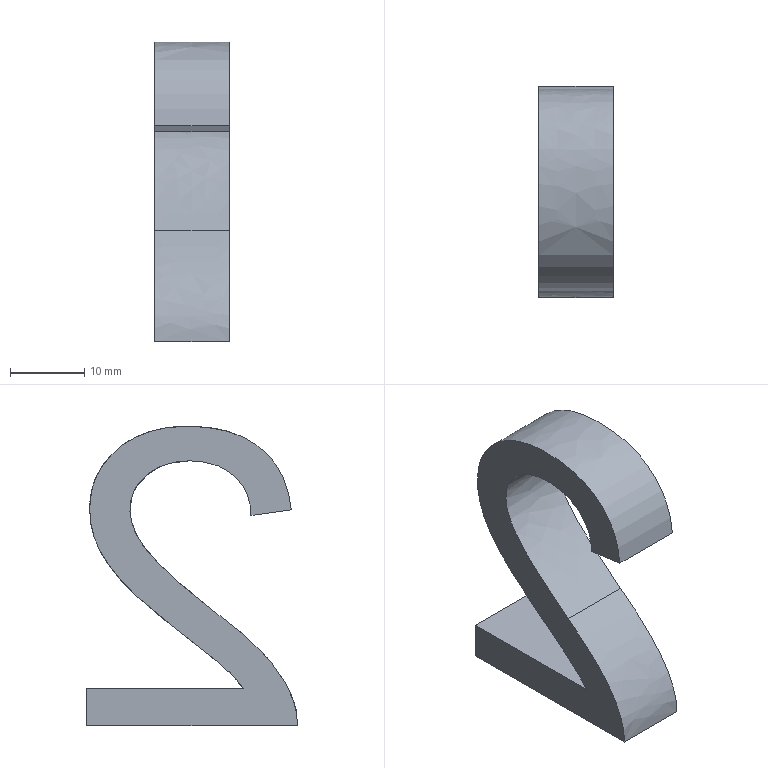Part | NX | features solid 2 | 1 solid | 10 faces | box 10 x 28.457 x 40.383 mm | volume 4760 mm3 | plane 6 | spline 4
STEP:
#1=CARTESIAN_POINT('',(2250.,-328.928,-584.952));
#2=VERTEX_POINT('',#1);
#3=CARTESIAN_POINT('',(2250.,-307.743,-584.952));
#4=VERTEX_POINT('',#3);
#5=CARTESIAN_POINT('',(2250.,-328.928,-584.952));
#6=CARTESIAN_POINT('',(2250.,-321.866,-584.952));
#7=CARTESIAN_POINT('',(2250.,-314.804,-584.952));
#8=CARTESIAN_POINT('',(2250.,-307.743,-584.952));
#9=B_SPLINE_CURVE_WITH_KNOTS('',3,(#5,#6,#7,#8),.UNSPECIFIED.,.F.,.F.,(4,4),(0.,0.09593),.PIECEWISE_BEZIER_KNOTS.);
#10=EDGE_CURVE('',#2,#4,#9,.T.);
#11=ORIENTED_EDGE('',*,*,#10,.F.);
#12=CARTESIAN_POINT('',(2260.,-328.928,-584.952));
#13=VERTEX_POINT('',#12);
#14=CARTESIAN_POINT('',(2260.,-328.928,-584.952));
#15=DIRECTION('',(-1.,0.,0.));
#16=VECTOR('',#15,1000.);
#17=LINE('',#14,#16);
#18=EDGE_CURVE('',#13,#2,#17,.T.);
#19=ORIENTED_EDGE('',*,*,#18,.F.);
#20=CARTESIAN_POINT('',(2260.,-307.743,-584.952));
#21=VERTEX_POINT('',#20);
#22=CARTESIAN_POINT('',(2260.,-328.928,-584.952));
#23=CARTESIAN_POINT('',(2260.,-321.866,-584.952));
#24=CARTESIAN_POINT('',(2260.,-314.804,-584.952));
#25=CARTESIAN_POINT('',(2260.,-307.743,-584.952));
#26=B_SPLINE_CURVE_WITH_KNOTS('',3,(#22,#23,#24,#25),.UNSPECIFIED.,.F.,.F.,(4,4),(0.,0.09593),.PIECEWISE_BEZIER_KNOTS.);
#27=EDGE_CURVE('',#13,#21,#26,.T.);
#28=ORIENTED_EDGE('',*,*,#27,.T.);
#29=CARTESIAN_POINT('',(2260.,-307.743,-584.952));
#30=DIRECTION('',(-1.,0.,0.));
#31=VECTOR('',#30,1000.);
#32=LINE('',#29,#31);
#33=EDGE_CURVE('',#21,#4,#32,.T.);
#34=ORIENTED_EDGE('',*,*,#33,.T.);
#35=EDGE_LOOP('',(#11,#19,#28,#34));
#36=FACE_BOUND('',#35,.T.);
#37=CARTESIAN_POINT('',(2260.,-328.928,-584.952));
#38=DIRECTION('',(0.,0.,1.));
#39=DIRECTION('',(1.,0.,0.));
#40=AXIS2_PLACEMENT_3D('',#37,#38,#39);
#41=PLANE('',#40);
#42=ADVANCED_FACE('',(#36),#41,.T.);
#43=CARTESIAN_POINT('',(2250.,-307.743,-590.));
#44=VERTEX_POINT('',#43);
#45=CARTESIAN_POINT('',(2250.,-307.743,-584.952));
#46=CARTESIAN_POINT('',(2250.,-307.743,-586.635));
#47=CARTESIAN_POINT('',(2250.,-307.743,-588.317));
#48=CARTESIAN_POINT('',(2250.,-307.743,-590.));
#49=B_SPLINE_CURVE_WITH_KNOTS('',3,(#45,#46,#47,#48),.UNSPECIFIED.,.F.,.F.,(4,4),(0.09593,0.1188),.PIECEWISE_BEZIER_KNOTS.);
#50=EDGE_CURVE('',#4,#44,#49,.T.);
#51=ORIENTED_EDGE('',*,*,#50,.F.);
#52=ORIENTED_EDGE('',*,*,#33,.F.);
#53=CARTESIAN_POINT('',(2260.,-307.743,-590.));
#54=VERTEX_POINT('',#53);
#55=CARTESIAN_POINT('',(2260.,-307.743,-584.952));
#56=CARTESIAN_POINT('',(2260.,-307.743,-586.635));
#57=CARTESIAN_POINT('',(2260.,-307.743,-588.317));
#58=CARTESIAN_POINT('',(2260.,-307.743,-590.));
#59=B_SPLINE_CURVE_WITH_KNOTS('',3,(#55,#56,#57,#58),.UNSPECIFIED.,.F.,.F.,(4,4),(0.09593,0.1188),.PIECEWISE_BEZIER_KNOTS.);
#60=EDGE_CURVE('',#21,#54,#59,.T.);
#61=ORIENTED_EDGE('',*,*,#60,.T.);
#62=CARTESIAN_POINT('',(2260.,-307.743,-590.));
#63=DIRECTION('',(-1.,0.,0.));
#64=VECTOR('',#63,1000.);
#65=LINE('',#62,#64);
#66=EDGE_CURVE('',#54,#44,#65,.T.);
#67=ORIENTED_EDGE('',*,*,#66,.T.);
#68=EDGE_LOOP('',(#51,#52,#61,#67));
#69=FACE_BOUND('',#68,.T.);
#70=CARTESIAN_POINT('',(2260.,-307.743,-584.952));
#71=DIRECTION('',(0.,1.,0.));
#72=DIRECTION('',(-1.,0.,0.));
#73=AXIS2_PLACEMENT_3D('',#70,#71,#72);
#74=PLANE('',#73);
#75=ADVANCED_FACE('',(#69),#74,.T.);
#76=CARTESIAN_POINT('',(2250.,-336.194,-590.));
#77=VERTEX_POINT('',#76);
#78=CARTESIAN_POINT('',(2250.,-307.743,-590.));
#79=CARTESIAN_POINT('',(2250.,-317.226,-590.));
#80=CARTESIAN_POINT('',(2250.,-326.71,-590.));
#81=CARTESIAN_POINT('',(2250.,-336.194,-590.));
#82=B_SPLINE_CURVE_WITH_KNOTS('',3,(#78,#79,#80,#81),.UNSPECIFIED.,.F.,.F.,(4,4),(0.1188,0.2476),.PIECEWISE_BEZIER_KNOTS.);
#83=EDGE_CURVE('',#44,#77,#82,.T.);
#84=ORIENTED_EDGE('',*,*,#83,.F.);
#85=ORIENTED_EDGE('',*,*,#66,.F.);
#86=CARTESIAN_POINT('',(2260.,-336.194,-590.));
#87=VERTEX_POINT('',#86);
#88=CARTESIAN_POINT('',(2260.,-307.743,-590.));
#89=CARTESIAN_POINT('',(2260.,-317.226,-590.));
#90=CARTESIAN_POINT('',(2260.,-326.71,-590.));
#91=CARTESIAN_POINT('',(2260.,-336.194,-590.));
#92=B_SPLINE_CURVE_WITH_KNOTS('',3,(#88,#89,#90,#91),.UNSPECIFIED.,.F.,.F.,(4,4),(0.1188,0.2476),.PIECEWISE_BEZIER_KNOTS.);
#93=EDGE_CURVE('',#54,#87,#92,.T.);
#94=ORIENTED_EDGE('',*,*,#93,.T.);
#95=CARTESIAN_POINT('',(2260.,-336.194,-590.));
#96=DIRECTION('',(-1.,0.,0.));
#97=VECTOR('',#96,1000.);
#98=LINE('',#95,#97);
#99=EDGE_CURVE('',#87,#77,#98,.T.);
#100=ORIENTED_EDGE('',*,*,#99,.T.);
#101=EDGE_LOOP('',(#84,#85,#94,#100));
#102=FACE_BOUND('',#101,.T.);
#103=CARTESIAN_POINT('',(2260.,-307.743,-590.));
#104=DIRECTION('',(0.,0.,-1.));
#105=DIRECTION('',(-1.,0.,0.));
#106=AXIS2_PLACEMENT_3D('',#103,#104,#105);
#107=PLANE('',#106);
#108=ADVANCED_FACE('',(#102),#107,.T.);
#109=CARTESIAN_POINT('',(2250.,-325.471,-574.979));
#110=VERTEX_POINT('',#109);
#111=CARTESIAN_POINT('',(2250.,-336.194,-590.));
#112=CARTESIAN_POINT('',(2250.,-336.24,-588.792));
#113=CARTESIAN_POINT('',(2250.,-336.026,-587.629));
#114=CARTESIAN_POINT('',(2250.,-335.597,-586.472));
#115=CARTESIAN_POINT('',(2250.,-334.909,-584.616));
#116=CARTESIAN_POINT('',(2250.,-333.777,-582.795));
#117=CARTESIAN_POINT('',(2250.,-332.239,-581.013));
#118=CARTESIAN_POINT('',(2250.,-330.702,-579.231));
#119=CARTESIAN_POINT('',(2250.,-328.454,-577.212));
#120=CARTESIAN_POINT('',(2250.,-325.471,-574.979));
#121=B_SPLINE_CURVE_WITH_KNOTS('',3,(#111,#112,#113,#114,#115,#116,#117,#118,#119,#120),.UNSPECIFIED.,.F.,.F.,(4,3,3,4),(0.2476,0.2639,0.2931,0.3343),.PIECEWISE_BEZIER_KNOTS.);
#122=EDGE_CURVE('',#77,#110,#121,.T.);
#123=ORIENTED_EDGE('',*,*,#122,.F.);
#124=ORIENTED_EDGE('',*,*,#99,.F.);
#125=CARTESIAN_POINT('',(2260.,-325.471,-574.979));
#126=VERTEX_POINT('',#125);
#127=CARTESIAN_POINT('',(2260.,-336.194,-590.));
#128=CARTESIAN_POINT('',(2260.,-336.24,-588.792));
#129=CARTESIAN_POINT('',(2260.,-336.026,-587.629));
#130=CARTESIAN_POINT('',(2260.,-335.597,-586.472));
#131=CARTESIAN_POINT('',(2260.,-334.909,-584.616));
#132=CARTESIAN_POINT('',(2260.,-333.777,-582.795));
#133=CARTESIAN_POINT('',(2260.,-332.239,-581.013));
#134=CARTESIAN_POINT('',(2260.,-330.702,-579.231));
#135=CARTESIAN_POINT('',(2260.,-328.454,-577.212));
#136=CARTESIAN_POINT('',(2260.,-325.471,-574.979));
#137=B_SPLINE_CURVE_WITH_KNOTS('',3,(#127,#128,#129,#130,#131,#132,#133,#134,#135,#136),.UNSPECIFIED.,.F.,.F.,(4,3,3,4),(0.2476,0.2639,0.2931,0.3343),.PIECEWISE_BEZIER_KNOTS.);
#138=EDGE_CURVE('',#87,#126,#137,.T.);
#139=ORIENTED_EDGE('',*,*,#138,.T.);
#140=CARTESIAN_POINT('',(2260.,-325.471,-574.979));
#141=DIRECTION('',(-1.,0.,0.));
#142=VECTOR('',#141,1000.);
#143=LINE('',#140,#142);
#144=EDGE_CURVE('',#126,#110,#143,.T.);
#145=ORIENTED_EDGE('',*,*,#144,.T.);
#146=EDGE_LOOP('',(#123,#124,#139,#145));
#147=FACE_BOUND('',#146,.T.);
#148=CARTESIAN_POINT('',(2260.,-336.194,-590.));
#149=CARTESIAN_POINT('',(2250.,-336.194,-590.));
#150=CARTESIAN_POINT('',(2260.,-336.224,-589.198));
#151=CARTESIAN_POINT('',(2250.,-336.224,-589.198));
#152=CARTESIAN_POINT('',(2260.,-336.108,-588.045));
#153=CARTESIAN_POINT('',(2250.,-336.108,-588.045));
#154=CARTESIAN_POINT('',(2260.,-335.61,-586.454));
#155=CARTESIAN_POINT('',(2250.,-335.61,-586.454));
#156=CARTESIAN_POINT('',(2260.,-335.051,-585.129));
#157=CARTESIAN_POINT('',(2250.,-335.051,-585.129));
#158=CARTESIAN_POINT('',(2260.,-334.296,-583.751));
#159=CARTESIAN_POINT('',(2250.,-334.296,-583.751));
#160=CARTESIAN_POINT('',(2260.,-333.371,-582.412));
#161=CARTESIAN_POINT('',(2250.,-333.371,-582.412));
#162=CARTESIAN_POINT('',(2260.,-332.723,-581.58));
#163=CARTESIAN_POINT('',(2250.,-332.723,-581.58));
#164=CARTESIAN_POINT('',(2260.,-332.157,-580.915));
#165=CARTESIAN_POINT('',(2250.,-332.157,-580.915));
#166=CARTESIAN_POINT('',(2260.,-331.777,-580.489));
#167=CARTESIAN_POINT('',(2250.,-331.777,-580.489));
#168=CARTESIAN_POINT('',(2260.,-330.948,-579.606));
#169=CARTESIAN_POINT('',(2250.,-330.948,-579.606));
#170=CARTESIAN_POINT('',(2260.,-329.1,-577.839));
#171=CARTESIAN_POINT('',(2250.,-329.1,-577.839));
#172=CARTESIAN_POINT('',(2260.,-327.042,-576.155));
#173=CARTESIAN_POINT('',(2250.,-327.042,-576.155));
#174=CARTESIAN_POINT('',(2260.,-325.471,-574.979));
#175=CARTESIAN_POINT('',(2250.,-325.471,-574.979));
#176=B_SPLINE_SURFACE_WITH_KNOTS('',3,1,((#148,#149),(#150,#151),(#152,#153),(#154,#155),(#156,#157),(#158,#159),(#160,#161),(#162,#163),(#164,#165),(#166,#167),(#168,#169),(#170,#171),(#172,#173),(#174,#175)),.SURF_OF_LINEAR_EXTRUSION.,.F.,.F.,.F.,(4,1,1,1,1,1,1,1,1,1,1,4),(2,2),(0.2476,0.2585,0.2639,0.2693,0.2801,0.2855,0.2909,0.2937,0.2964,0.3018,0.3126,0.3343),(0.,1.),.UNSPECIFIED.);
#177=ADVANCED_FACE('',(#147),#176,.T.);
#178=CARTESIAN_POINT('',(2250.,-321.601,-554.268));
#179=VERTEX_POINT('',#178);
#180=CARTESIAN_POINT('',(2250.,-325.471,-574.979));
#181=CARTESIAN_POINT('',(2250.,-320.852,-571.415));
#182=CARTESIAN_POINT('',(2250.,-317.701,-568.616));
#183=CARTESIAN_POINT('',(2250.,-314.421,-564.631));
#184=CARTESIAN_POINT('',(2250.,-313.601,-562.727));
#185=CARTESIAN_POINT('',(2250.,-313.601,-559.055));
#186=CARTESIAN_POINT('',(2250.,-314.335,-557.511));
#187=CARTESIAN_POINT('',(2250.,-315.827,-556.22));
#188=CARTESIAN_POINT('',(2250.,-317.288,-554.956));
#189=CARTESIAN_POINT('',(2250.,-319.23,-554.298));
#190=CARTESIAN_POINT('',(2250.,-321.601,-554.268));
#191=B_SPLINE_CURVE_WITH_KNOTS('',3,(#180,#181,#182,#183,#184,#185,#186,#187,#188,#189,#190),.UNSPECIFIED.,.F.,.F.,(4,2,2,3,4),(0.3343,0.3913,0.4486,0.5049,0.537),.UNSPECIFIED.);
#192=EDGE_CURVE('',#110,#179,#191,.T.);
#193=ORIENTED_EDGE('',*,*,#192,.F.);
#194=ORIENTED_EDGE('',*,*,#144,.F.);
#195=CARTESIAN_POINT('',(2260.,-321.601,-554.268));
#196=VERTEX_POINT('',#195);
#197=CARTESIAN_POINT('',(2260.,-325.471,-574.979));
#198=CARTESIAN_POINT('',(2260.,-320.852,-571.415));
#199=CARTESIAN_POINT('',(2260.,-317.701,-568.616));
#200=CARTESIAN_POINT('',(2260.,-314.421,-564.631));
#201=CARTESIAN_POINT('',(2260.,-313.601,-562.727));
#202=CARTESIAN_POINT('',(2260.,-313.601,-559.055));
#203=CARTESIAN_POINT('',(2260.,-314.335,-557.511));
#204=CARTESIAN_POINT('',(2260.,-315.827,-556.22));
#205=CARTESIAN_POINT('',(2260.,-317.288,-554.956));
#206=CARTESIAN_POINT('',(2260.,-319.23,-554.298));
#207=CARTESIAN_POINT('',(2260.,-321.601,-554.268));
#208=B_SPLINE_CURVE_WITH_KNOTS('',3,(#197,#198,#199,#200,#201,#202,#203,#204,#205,#206,#207),.UNSPECIFIED.,.F.,.F.,(4,2,2,3,4),(0.3343,0.3913,0.4486,0.5049,0.537),.UNSPECIFIED.);
#209=EDGE_CURVE('',#126,#196,#208,.T.);
#210=ORIENTED_EDGE('',*,*,#209,.T.);
#211=CARTESIAN_POINT('',(2260.,-321.601,-554.268));
#212=DIRECTION('',(-1.,0.,0.));
#213=VECTOR('',#212,1000.);
#214=LINE('',#211,#213);
#215=EDGE_CURVE('',#196,#179,#214,.T.);
#216=ORIENTED_EDGE('',*,*,#215,.T.);
#217=EDGE_LOOP('',(#193,#194,#210,#216));
#218=FACE_BOUND('',#217,.T.);
#219=CARTESIAN_POINT('',(2260.,-325.471,-574.979));
#220=CARTESIAN_POINT('',(2250.,-325.471,-574.979));
#221=CARTESIAN_POINT('',(2260.,-323.42,-573.396));
#222=CARTESIAN_POINT('',(2250.,-323.42,-573.396));
#223=CARTESIAN_POINT('',(2260.,-319.899,-570.535));
#224=CARTESIAN_POINT('',(2250.,-319.899,-570.535));
#225=CARTESIAN_POINT('',(2260.,-316.953,-567.72));
#226=CARTESIAN_POINT('',(2250.,-316.953,-567.72));
#227=CARTESIAN_POINT('',(2260.,-315.515,-565.972));
#228=CARTESIAN_POINT('',(2250.,-315.515,-565.972));
#229=CARTESIAN_POINT('',(2260.,-314.378,-564.235));
#230=CARTESIAN_POINT('',(2250.,-314.378,-564.235));
#231=CARTESIAN_POINT('',(2260.,-313.566,-562.136));
#232=CARTESIAN_POINT('',(2250.,-313.566,-562.136));
#233=CARTESIAN_POINT('',(2260.,-313.559,-559.658));
#234=CARTESIAN_POINT('',(2250.,-313.559,-559.658));
#235=CARTESIAN_POINT('',(2260.,-314.22,-558.066));
#236=CARTESIAN_POINT('',(2250.,-314.22,-558.066));
#237=CARTESIAN_POINT('',(2260.,-314.95,-557.098));
#238=CARTESIAN_POINT('',(2250.,-314.95,-557.098));
#239=CARTESIAN_POINT('',(2260.,-315.295,-556.715));
#240=CARTESIAN_POINT('',(2250.,-315.295,-556.715));
#241=CARTESIAN_POINT('',(2260.,-315.614,-556.409));
#242=CARTESIAN_POINT('',(2250.,-315.614,-556.409));
#243=CARTESIAN_POINT('',(2260.,-315.829,-556.211));
#244=CARTESIAN_POINT('',(2250.,-315.829,-556.211));
#245=CARTESIAN_POINT('',(2260.,-316.335,-555.807));
#246=CARTESIAN_POINT('',(2250.,-316.335,-555.807));
#247=CARTESIAN_POINT('',(2260.,-316.954,-555.401));
#248=CARTESIAN_POINT('',(2250.,-316.954,-555.401));
#249=CARTESIAN_POINT('',(2260.,-317.83,-554.954));
#250=CARTESIAN_POINT('',(2250.,-317.83,-554.954));
#251=CARTESIAN_POINT('',(2260.,-319.356,-554.446));
#252=CARTESIAN_POINT('',(2250.,-319.356,-554.446));
#253=CARTESIAN_POINT('',(2260.,-320.664,-554.28));
#254=CARTESIAN_POINT('',(2250.,-320.664,-554.28));
#255=CARTESIAN_POINT('',(2260.,-321.601,-554.268));
#256=CARTESIAN_POINT('',(2250.,-321.601,-554.268));
#257=B_SPLINE_SURFACE_WITH_KNOTS('',3,1,((#219,#220),(#221,#222),(#223,#224),(#225,#226),(#227,#228),(#229,#230),(#231,#232),(#233,#234),(#235,#236),(#237,#238),(#239,#240),(#241,#242),(#243,#244),(#245,#246),(#247,#248),(#249,#250),(#251,#252),(#253,#254),(#255,#256)),.SURF_OF_LINEAR_EXTRUSION.,.F.,.F.,.F.,(4,1,1,1,1,1,1,1,1,1,1,1,1,1,1,1,4),(2,2),(0.3343,0.3596,0.3849,0.3976,0.4103,0.4356,0.461,0.4863,0.4926,0.499,0.5021,0.5053,0.5085,0.5116,0.518,0.5243,0.537),(0.,1.),.UNSPECIFIED.);
#258=ADVANCED_FACE('',(#218),#257,.T.);
#259=CARTESIAN_POINT('',(2250.,-329.922,-561.656));
#260=VERTEX_POINT('',#259);
#261=CARTESIAN_POINT('',(2250.,-321.601,-554.268));
#262=CARTESIAN_POINT('',(2250.,-324.11,-554.298));
#263=CARTESIAN_POINT('',(2250.,-326.098,-554.956));
#264=CARTESIAN_POINT('',(2250.,-329.119,-557.58));
#265=CARTESIAN_POINT('',(2250.,-329.892,-559.377));
#266=CARTESIAN_POINT('',(2250.,-329.922,-561.656));
#267=B_SPLINE_CURVE_WITH_KNOTS('',3,(#261,#262,#263,#264,#265,#266),.UNSPECIFIED.,.F.,.F.,(4,2,4),(0.537,0.5703,0.6034),.UNSPECIFIED.);
#268=EDGE_CURVE('',#179,#260,#267,.T.);
#269=ORIENTED_EDGE('',*,*,#268,.F.);
#270=ORIENTED_EDGE('',*,*,#215,.F.);
#271=CARTESIAN_POINT('',(2260.,-329.922,-561.656));
#272=VERTEX_POINT('',#271);
#273=CARTESIAN_POINT('',(2260.,-321.601,-554.268));
#274=CARTESIAN_POINT('',(2260.,-324.11,-554.298));
#275=CARTESIAN_POINT('',(2260.,-326.098,-554.956));
#276=CARTESIAN_POINT('',(2260.,-329.119,-557.58));
#277=CARTESIAN_POINT('',(2260.,-329.892,-559.377));
#278=CARTESIAN_POINT('',(2260.,-329.922,-561.656));
#279=B_SPLINE_CURVE_WITH_KNOTS('',3,(#273,#274,#275,#276,#277,#278),.UNSPECIFIED.,.F.,.F.,(4,2,4),(0.537,0.5703,0.6034),.UNSPECIFIED.);
#280=EDGE_CURVE('',#196,#272,#279,.T.);
#281=ORIENTED_EDGE('',*,*,#280,.T.);
#282=CARTESIAN_POINT('',(2260.,-329.922,-561.656));
#283=DIRECTION('',(-1.,0.,0.));
#284=VECTOR('',#283,1000.);
#285=LINE('',#282,#284);
#286=EDGE_CURVE('',#272,#260,#285,.T.);
#287=ORIENTED_EDGE('',*,*,#286,.T.);
#288=EDGE_LOOP('',(#269,#270,#281,#287));
#289=FACE_BOUND('',#288,.T.);
#290=CARTESIAN_POINT('',(2260.,-321.601,-554.268));
#291=CARTESIAN_POINT('',(2250.,-321.601,-554.268));
#292=CARTESIAN_POINT('',(2260.,-322.852,-554.283));
#293=CARTESIAN_POINT('',(2250.,-322.852,-554.283));
#294=CARTESIAN_POINT('',(2260.,-325.087,-554.62));
#295=CARTESIAN_POINT('',(2250.,-325.087,-554.62));
#296=CARTESIAN_POINT('',(2260.,-327.752,-556.118));
#297=CARTESIAN_POINT('',(2250.,-327.752,-556.118));
#298=CARTESIAN_POINT('',(2260.,-329.513,-558.477));
#299=CARTESIAN_POINT('',(2250.,-329.513,-558.477));
#300=CARTESIAN_POINT('',(2260.,-329.907,-560.513));
#301=CARTESIAN_POINT('',(2250.,-329.907,-560.513));
#302=CARTESIAN_POINT('',(2260.,-329.922,-561.656));
#303=CARTESIAN_POINT('',(2250.,-329.922,-561.656));
#304=B_SPLINE_SURFACE_WITH_KNOTS('',3,1,((#290,#291),(#292,#293),(#294,#295),(#296,#297),(#298,#299),(#300,#301),(#302,#303)),.SURF_OF_LINEAR_EXTRUSION.,.F.,.F.,.F.,(4,1,1,1,4),(2,2),(0.537,0.5536,0.5702,0.5868,0.6034),(0.,1.),.UNSPECIFIED.);
#305=ADVANCED_FACE('',(#289),#304,.T.);
#306=CARTESIAN_POINT('',(2250.,-335.353,-560.876));
#307=VERTEX_POINT('',#306);
#308=CARTESIAN_POINT('',(2250.,-329.922,-561.656));
#309=CARTESIAN_POINT('',(2250.,-331.732,-561.396));
#310=CARTESIAN_POINT('',(2250.,-333.543,-561.136));
#311=CARTESIAN_POINT('',(2250.,-335.353,-560.876));
#312=B_SPLINE_CURVE_WITH_KNOTS('',3,(#308,#309,#310,#311),.UNSPECIFIED.,.F.,.F.,(4,4),(0.6034,0.6317),.PIECEWISE_BEZIER_KNOTS.);
#313=EDGE_CURVE('',#260,#307,#312,.T.);
#314=ORIENTED_EDGE('',*,*,#313,.F.);
#315=ORIENTED_EDGE('',*,*,#286,.F.);
#316=CARTESIAN_POINT('',(2260.,-335.353,-560.876));
#317=VERTEX_POINT('',#316);
#318=CARTESIAN_POINT('',(2260.,-329.922,-561.656));
#319=CARTESIAN_POINT('',(2260.,-331.732,-561.396));
#320=CARTESIAN_POINT('',(2260.,-333.543,-561.136));
#321=CARTESIAN_POINT('',(2260.,-335.353,-560.876));
#322=B_SPLINE_CURVE_WITH_KNOTS('',3,(#318,#319,#320,#321),.UNSPECIFIED.,.F.,.F.,(4,4),(0.6034,0.6317),.PIECEWISE_BEZIER_KNOTS.);
#323=EDGE_CURVE('',#272,#317,#322,.T.);
#324=ORIENTED_EDGE('',*,*,#323,.T.);
#325=CARTESIAN_POINT('',(2260.,-335.353,-560.876));
#326=DIRECTION('',(-1.,0.,0.));
#327=VECTOR('',#326,1000.);
#328=LINE('',#325,#327);
#329=EDGE_CURVE('',#317,#307,#328,.T.);
#330=ORIENTED_EDGE('',*,*,#329,.T.);
#331=EDGE_LOOP('',(#314,#315,#324,#330));
#332=FACE_BOUND('',#331,.T.);
#333=CARTESIAN_POINT('',(2260.,-329.922,-561.656));
#334=DIRECTION('',(0.,-0.1422,-0.9898));
#335=DIRECTION('',(0.,0.9898,-0.1422));
#336=AXIS2_PLACEMENT_3D('',#333,#334,#335);
#337=PLANE('',#336);
#338=ADVANCED_FACE('',(#332),#337,.T.);
#339=CARTESIAN_POINT('',(2250.,-335.353,-560.876));
#340=CARTESIAN_POINT('',(2250.,-334.985,-557.235));
#341=CARTESIAN_POINT('',(2250.,-333.594,-554.467));
#342=CARTESIAN_POINT('',(2250.,-328.805,-550.593));
#343=CARTESIAN_POINT('',(2250.,-325.548,-549.633));
#344=CARTESIAN_POINT('',(2250.,-317.395,-549.602));
#345=CARTESIAN_POINT('',(2250.,-314.152,-550.704));
#346=CARTESIAN_POINT('',(2250.,-309.341,-554.993));
#347=CARTESIAN_POINT('',(2250.,-308.171,-557.648));
#348=CARTESIAN_POINT('',(2250.,-308.171,-562.451));
#349=CARTESIAN_POINT('',(2250.,-308.477,-564.027));
#350=CARTESIAN_POINT('',(2250.,-309.851,-567.142));
#351=CARTESIAN_POINT('',(2250.,-310.94,-568.784));
#352=CARTESIAN_POINT('',(2250.,-312.488,-570.508));
#353=CARTESIAN_POINT('',(2250.,-314.045,-572.241));
#354=CARTESIAN_POINT('',(2250.,-316.691,-574.551));
#355=CARTESIAN_POINT('',(2250.,-323.601,-579.875));
#356=CARTESIAN_POINT('',(2250.,-325.655,-581.541));
#357=CARTESIAN_POINT('',(2250.,-326.584,-582.387));
#358=CARTESIAN_POINT('',(2250.,-327.536,-583.254));
#359=CARTESIAN_POINT('',(2250.,-328.301,-584.126));
#360=CARTESIAN_POINT('',(2250.,-328.928,-584.952));
#361=B_SPLINE_CURVE_WITH_KNOTS('',3,(#339,#340,#341,#342,#343,#344,#345,#346,#347,#348,#349,#350,#351,#352,#353,#354,#355,#356,#357,#358,#359,#360),.UNSPECIFIED.,.F.,.F.,(4,2,2,2,2,2,3,2,3,4),(0.6317,0.6813,0.7305,0.7802,0.8302,0.8563,0.8824,0.9363,0.9821,1.),.UNSPECIFIED.);
#362=EDGE_CURVE('',#307,#2,#361,.T.);
#363=ORIENTED_EDGE('',*,*,#362,.F.);
#364=ORIENTED_EDGE('',*,*,#329,.F.);
#365=CARTESIAN_POINT('',(2260.,-335.353,-560.876));
#366=CARTESIAN_POINT('',(2260.,-334.985,-557.235));
#367=CARTESIAN_POINT('',(2260.,-333.594,-554.467));
#368=CARTESIAN_POINT('',(2260.,-328.805,-550.593));
#369=CARTESIAN_POINT('',(2260.,-325.548,-549.633));
#370=CARTESIAN_POINT('',(2260.,-317.395,-549.602));
#371=CARTESIAN_POINT('',(2260.,-314.152,-550.704));
#372=CARTESIAN_POINT('',(2260.,-309.341,-554.993));
#373=CARTESIAN_POINT('',(2260.,-308.171,-557.648));
#374=CARTESIAN_POINT('',(2260.,-308.171,-562.451));
#375=CARTESIAN_POINT('',(2260.,-308.477,-564.027));
#376=CARTESIAN_POINT('',(2260.,-309.851,-567.142));
#377=CARTESIAN_POINT('',(2260.,-310.94,-568.784));
#378=CARTESIAN_POINT('',(2260.,-312.488,-570.508));
#379=CARTESIAN_POINT('',(2260.,-314.045,-572.241));
#380=CARTESIAN_POINT('',(2260.,-316.691,-574.551));
#381=CARTESIAN_POINT('',(2260.,-323.601,-579.875));
#382=CARTESIAN_POINT('',(2260.,-325.655,-581.541));
#383=CARTESIAN_POINT('',(2260.,-326.584,-582.387));
#384=CARTESIAN_POINT('',(2260.,-327.536,-583.254));
#385=CARTESIAN_POINT('',(2260.,-328.301,-584.126));
#386=CARTESIAN_POINT('',(2260.,-328.928,-584.952));
#387=B_SPLINE_CURVE_WITH_KNOTS('',3,(#365,#366,#367,#368,#369,#370,#371,#372,#373,#374,#375,#376,#377,#378,#379,#380,#381,#382,#383,#384,#385,#386),.UNSPECIFIED.,.F.,.F.,(4,2,2,2,2,2,3,2,3,4),(0.6317,0.6813,0.7305,0.7802,0.8302,0.8563,0.8824,0.9363,0.9821,1.),.UNSPECIFIED.);
#388=EDGE_CURVE('',#317,#13,#387,.T.);
#389=ORIENTED_EDGE('',*,*,#388,.T.);
#390=ORIENTED_EDGE('',*,*,#18,.T.);
#391=EDGE_LOOP('',(#363,#364,#389,#390));
#392=FACE_BOUND('',#391,.T.);
#393=CARTESIAN_POINT('',(2260.,-335.353,-560.876));
#394=CARTESIAN_POINT('',(2250.,-335.353,-560.876));
#395=CARTESIAN_POINT('',(2260.,-335.011,-557.491));
#396=CARTESIAN_POINT('',(2250.,-335.011,-557.491));
#397=CARTESIAN_POINT('',(2260.,-333.161,-553.526));
#398=CARTESIAN_POINT('',(2250.,-333.161,-553.526));
#399=CARTESIAN_POINT('',(2260.,-328.113,-550.464));
#400=CARTESIAN_POINT('',(2250.,-328.113,-550.464));
#401=CARTESIAN_POINT('',(2260.,-324.107,-549.639));
#402=CARTESIAN_POINT('',(2250.,-324.107,-549.639));
#403=CARTESIAN_POINT('',(2260.,-320.273,-549.585));
#404=CARTESIAN_POINT('',(2250.,-320.273,-549.585));
#405=CARTESIAN_POINT('',(2260.,-316.821,-550.01));
#406=CARTESIAN_POINT('',(2250.,-316.821,-550.01));
#407=CARTESIAN_POINT('',(2260.,-313.189,-551.406));
#408=CARTESIAN_POINT('',(2250.,-313.189,-551.406));
#409=CARTESIAN_POINT('',(2260.,-309.889,-554.485));
#410=CARTESIAN_POINT('',(2250.,-309.889,-554.485));
#411=CARTESIAN_POINT('',(2260.,-308.211,-558.084));
#412=CARTESIAN_POINT('',(2250.,-308.211,-558.084));
#413=CARTESIAN_POINT('',(2260.,-308.056,-561.745));
#414=CARTESIAN_POINT('',(2250.,-308.056,-561.745));
#415=CARTESIAN_POINT('',(2260.,-308.684,-564.528));
#416=CARTESIAN_POINT('',(2250.,-308.684,-564.528));
#417=CARTESIAN_POINT('',(2260.,-309.581,-566.578));
#418=CARTESIAN_POINT('',(2250.,-309.581,-566.578));
#419=CARTESIAN_POINT('',(2260.,-310.725,-568.371));
#420=CARTESIAN_POINT('',(2250.,-310.725,-568.371));
#421=CARTESIAN_POINT('',(2260.,-311.695,-569.592));
#422=CARTESIAN_POINT('',(2250.,-311.695,-569.592));
#423=CARTESIAN_POINT('',(2260.,-312.166,-570.144));
#424=CARTESIAN_POINT('',(2250.,-312.166,-570.144));
#425=CARTESIAN_POINT('',(2260.,-312.535,-570.562));
#426=CARTESIAN_POINT('',(2250.,-312.535,-570.562));
#427=CARTESIAN_POINT('',(2260.,-312.696,-570.737));
#428=CARTESIAN_POINT('',(2250.,-312.696,-570.737));
#429=CARTESIAN_POINT('',(2260.,-312.988,-571.047));
#430=CARTESIAN_POINT('',(2250.,-312.988,-571.047));
#431=CARTESIAN_POINT('',(2260.,-313.374,-571.442));
#432=CARTESIAN_POINT('',(2250.,-313.374,-571.442));
#433=CARTESIAN_POINT('',(2260.,-313.913,-571.972));
#434=CARTESIAN_POINT('',(2250.,-313.913,-571.972));
#435=CARTESIAN_POINT('',(2260.,-314.63,-572.642));
#436=CARTESIAN_POINT('',(2250.,-314.63,-572.642));
#437=CARTESIAN_POINT('',(2260.,-315.687,-573.59));
#438=CARTESIAN_POINT('',(2250.,-315.687,-573.59));
#439=CARTESIAN_POINT('',(2260.,-317.196,-574.873));
#440=CARTESIAN_POINT('',(2250.,-317.196,-574.873));
#441=CARTESIAN_POINT('',(2260.,-319.292,-576.561));
#442=CARTESIAN_POINT('',(2250.,-319.292,-576.561));
#443=CARTESIAN_POINT('',(2260.,-321.734,-578.434));
#444=CARTESIAN_POINT('',(2250.,-321.734,-578.434));
#445=CARTESIAN_POINT('',(2260.,-323.668,-579.958));
#446=CARTESIAN_POINT('',(2250.,-323.668,-579.958));
#447=CARTESIAN_POINT('',(2260.,-324.945,-580.99));
#448=CARTESIAN_POINT('',(2250.,-324.945,-580.99));
#449=CARTESIAN_POINT('',(2260.,-325.748,-581.657));
#450=CARTESIAN_POINT('',(2250.,-325.748,-581.657));
#451=CARTESIAN_POINT('',(2260.,-326.169,-582.018));
#452=CARTESIAN_POINT('',(2250.,-326.169,-582.018));
#453=CARTESIAN_POINT('',(2260.,-326.401,-582.223));
#454=CARTESIAN_POINT('',(2250.,-326.401,-582.223));
#455=CARTESIAN_POINT('',(2260.,-326.528,-582.336));
#456=CARTESIAN_POINT('',(2250.,-326.528,-582.336));
#457=CARTESIAN_POINT('',(2260.,-326.562,-582.367));
#458=CARTESIAN_POINT('',(2250.,-326.562,-582.367));
#459=CARTESIAN_POINT('',(2260.,-326.805,-582.589));
#460=CARTESIAN_POINT('',(2250.,-326.805,-582.589));
#461=CARTESIAN_POINT('',(2260.,-327.123,-582.894));
#462=CARTESIAN_POINT('',(2250.,-327.123,-582.894));
#463=CARTESIAN_POINT('',(2260.,-327.676,-583.455));
#464=CARTESIAN_POINT('',(2250.,-327.676,-583.455));
#465=CARTESIAN_POINT('',(2260.,-328.294,-584.145));
#466=CARTESIAN_POINT('',(2250.,-328.294,-584.145));
#467=CARTESIAN_POINT('',(2260.,-328.726,-584.686));
#468=CARTESIAN_POINT('',(2250.,-328.726,-584.686));
#469=CARTESIAN_POINT('',(2260.,-328.928,-584.952));
#470=CARTESIAN_POINT('',(2250.,-328.928,-584.952));
#471=B_SPLINE_SURFACE_WITH_KNOTS('',3,1,((#393,#394),(#395,#396),(#397,#398),(#399,#400),(#401,#402),(#403,#404),(#405,#406),(#407,#408),(#409,#410),(#411,#412),(#413,#414),(#415,#416),(#417,#418),(#419,#420),(#421,#422),(#423,#424),(#425,#426),(#427,#428),(#429,#430),(#431,#432),(#433,#434),(#435,#436),(#437,#438),(#439,#440),(#441,#442),(#443,#444),(#445,#446),(#447,#448),(#449,#450),(#451,#452),(#453,#454),(#455,#456),(#457,#458),(#459,#460),(#461,#462),(#463,#464),(#465,#466),(#467,#468),(#469,#470)),.SURF_OF_LINEAR_EXTRUSION.,.F.,.F.,.F.,(4,1,1,1,1,1,1,1,1,1,1,1,1,1,1,1,1,1,1,1,1,1,1,1,1,1,1,1,1,1,1,1,1,1,1,1,4),(2,2),(0.6317,0.6778,0.7008,0.7238,0.7353,0.7468,0.7698,0.7929,0.8159,0.8389,0.8504,0.8619,0.8734,0.8792,0.8806,0.882,0.8849,0.8878,0.8907,0.8964,0.9022,0.9079,0.9194,0.931,0.9425,0.954,0.9655,0.9712,0.977,0.9799,0.9813,0.982,0.9827,0.9856,0.9885,0.9942,1.),(0.,1.),.UNSPECIFIED.);
#472=ADVANCED_FACE('',(#392),#471,.T.);
#473=ORIENTED_EDGE('',*,*,#27,.F.);
#474=ORIENTED_EDGE('',*,*,#388,.F.);
#475=ORIENTED_EDGE('',*,*,#323,.F.);
#476=ORIENTED_EDGE('',*,*,#280,.F.);
#477=ORIENTED_EDGE('',*,*,#209,.F.);
#478=ORIENTED_EDGE('',*,*,#138,.F.);
#479=ORIENTED_EDGE('',*,*,#93,.F.);
#480=ORIENTED_EDGE('',*,*,#60,.F.);
#481=EDGE_LOOP('',(#473,#474,#475,#476,#477,#478,#479,#480));
#482=FACE_BOUND('',#481,.T.);
#483=CARTESIAN_POINT('',(2260.,-332.578,-581.414));
#484=DIRECTION('',(1.,0.,0.));
#485=DIRECTION('',(0.,1.,0.));
#486=AXIS2_PLACEMENT_3D('',#483,#484,#485);
#487=PLANE('',#486);
#488=ADVANCED_FACE('',(#482),#487,.T.);
#489=ORIENTED_EDGE('',*,*,#10,.T.);
#490=ORIENTED_EDGE('',*,*,#50,.T.);
#491=ORIENTED_EDGE('',*,*,#83,.T.);
#492=ORIENTED_EDGE('',*,*,#122,.T.);
#493=ORIENTED_EDGE('',*,*,#192,.T.);
#494=ORIENTED_EDGE('',*,*,#268,.T.);
#495=ORIENTED_EDGE('',*,*,#313,.T.);
#496=ORIENTED_EDGE('',*,*,#362,.T.);
#497=EDGE_LOOP('',(#489,#490,#491,#492,#493,#494,#495,#496));
#498=FACE_BOUND('',#497,.T.);
#499=CARTESIAN_POINT('',(2250.,-332.578,-581.414));
#500=DIRECTION('',(1.,0.,0.));
#501=DIRECTION('',(0.,1.,0.));
#502=AXIS2_PLACEMENT_3D('',#499,#500,#501);
#503=PLANE('',#502);
#504=ADVANCED_FACE('',(#498),#503,.F.);
#505=CLOSED_SHELL('',(#42,#75,#108,#177,#258,#305,#338,#472,#488,#504));
#506=MANIFOLD_SOLID_BREP('',#505);
#507=(LENGTH_UNIT()NAMED_UNIT(*)SI_UNIT(.MILLI.,.METRE.));
#508=UNCERTAINTY_MEASURE_WITH_UNIT(LENGTH_MEASURE(0.0508),#507,'','');
#509=(NAMED_UNIT(*)PLANE_ANGLE_UNIT()SI_UNIT($,.RADIAN.));
#510=(NAMED_UNIT(*)SI_UNIT($,.STERADIAN.)SOLID_ANGLE_UNIT());
#511=(GEOMETRIC_REPRESENTATION_CONTEXT(3)GLOBAL_UNCERTAINTY_ASSIGNED_CONTEXT((#508))GLOBAL_UNIT_ASSIGNED_CONTEXT((#507,#509,#510))REPRESENTATION_CONTEXT('',''));
#512=ADVANCED_BREP_SHAPE_REPRESENTATION('',(#506),#511);